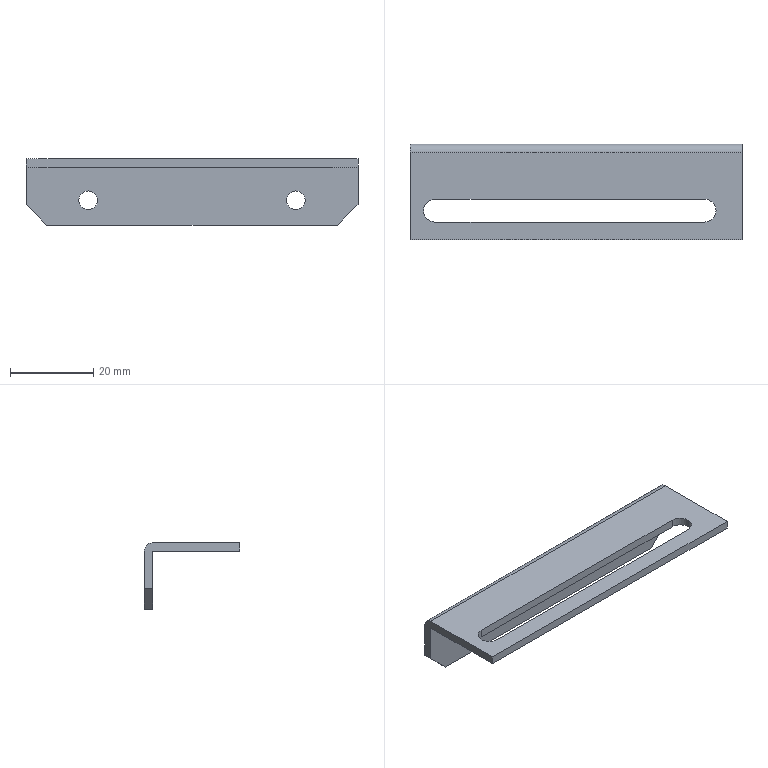Part | SolidWorks | features ICE 5, Chamfer 3, HoleWzd 3, Extrusion 1, Fillet 1 | 1 solid | 20 faces | box 80 x 23 x 16 mm | volume 4975 mm3 | plane 12 | cylinder 8 | commonest cylinder face diameters 4.5 x4 5.5 x3 4 x1
STEP:
#1=CARTESIAN_POINT('',(-10.,10.5,5.75));
#2=VERTEX_POINT('',#1);
#3=CARTESIAN_POINT('',(-10.,10.5,10.25));
#4=VERTEX_POINT('',#3);
#5=CARTESIAN_POINT('',(-10.,10.5,8.));
#6=DIRECTION('',(0.,1.,0.));
#7=DIRECTION('',(0.,0.,1.));
#8=AXIS2_PLACEMENT_3D('',#5,#6,#7);
#9=CIRCLE('',#8,2.25);
#10=EDGE_CURVE('',#2,#4,#9,.T.);
#11=ORIENTED_EDGE('',*,*,#10,.F.);
#12=CARTESIAN_POINT('',(-10.,12.5,5.75));
#13=VERTEX_POINT('',#12);
#14=CARTESIAN_POINT('',(-10.,12.5,5.75));
#15=DIRECTION('',(0.,1.,0.));
#16=VECTOR('',#15,1000.);
#17=LINE('',#14,#16);
#18=EDGE_CURVE('',#2,#13,#17,.T.);
#19=ORIENTED_EDGE('',*,*,#18,.T.);
#20=CARTESIAN_POINT('',(-10.,12.5,10.25));
#21=VERTEX_POINT('',#20);
#22=CARTESIAN_POINT('',(-10.,12.5,8.));
#23=DIRECTION('',(0.,1.,0.));
#24=DIRECTION('',(0.,0.,1.));
#25=AXIS2_PLACEMENT_3D('',#22,#23,#24);
#26=CIRCLE('',#25,2.25);
#27=EDGE_CURVE('',#13,#21,#26,.T.);
#28=ORIENTED_EDGE('',*,*,#27,.T.);
#29=CARTESIAN_POINT('',(-10.,12.5,10.25));
#30=DIRECTION('',(0.,1.,0.));
#31=VECTOR('',#30,1000.);
#32=LINE('',#29,#31);
#33=EDGE_CURVE('',#4,#21,#32,.T.);
#34=ORIENTED_EDGE('',*,*,#33,.F.);
#35=EDGE_LOOP('',(#11,#19,#28,#34));
#36=FACE_OUTER_BOUND('',#35,.T.);
#37=CARTESIAN_POINT('',(-10.,12.5,8.));
#38=DIRECTION('',(0.,1.,0.));
#39=DIRECTION('',(0.,0.,1.));
#40=AXIS2_PLACEMENT_3D('',#37,#38,#39);
#41=CYLINDRICAL_SURFACE('',#40,2.25);
#42=ADVANCED_FACE('',(#36),#41,.F.);
#43=CARTESIAN_POINT('',(-60.,10.5,5.75));
#44=VERTEX_POINT('',#43);
#45=CARTESIAN_POINT('',(-60.,10.5,10.25));
#46=VERTEX_POINT('',#45);
#47=CARTESIAN_POINT('',(-60.,10.5,8.));
#48=DIRECTION('',(0.,1.,0.));
#49=DIRECTION('',(0.,0.,1.));
#50=AXIS2_PLACEMENT_3D('',#47,#48,#49);
#51=CIRCLE('',#50,2.25);
#52=EDGE_CURVE('',#44,#46,#51,.T.);
#53=ORIENTED_EDGE('',*,*,#52,.F.);
#54=CARTESIAN_POINT('',(-60.,12.5,5.75));
#55=VERTEX_POINT('',#54);
#56=CARTESIAN_POINT('',(-60.,12.5,5.75));
#57=DIRECTION('',(0.,1.,0.));
#58=VECTOR('',#57,1000.);
#59=LINE('',#56,#58);
#60=EDGE_CURVE('',#44,#55,#59,.T.);
#61=ORIENTED_EDGE('',*,*,#60,.T.);
#62=CARTESIAN_POINT('',(-60.,12.5,10.25));
#63=VERTEX_POINT('',#62);
#64=CARTESIAN_POINT('',(-60.,12.5,8.));
#65=DIRECTION('',(0.,1.,0.));
#66=DIRECTION('',(0.,0.,1.));
#67=AXIS2_PLACEMENT_3D('',#64,#65,#66);
#68=CIRCLE('',#67,2.25);
#69=EDGE_CURVE('',#55,#63,#68,.T.);
#70=ORIENTED_EDGE('',*,*,#69,.T.);
#71=CARTESIAN_POINT('',(-60.,12.5,10.25));
#72=DIRECTION('',(0.,1.,0.));
#73=VECTOR('',#72,1000.);
#74=LINE('',#71,#73);
#75=EDGE_CURVE('',#46,#63,#74,.T.);
#76=ORIENTED_EDGE('',*,*,#75,.F.);
#77=EDGE_LOOP('',(#53,#61,#70,#76));
#78=FACE_OUTER_BOUND('',#77,.T.);
#79=CARTESIAN_POINT('',(-60.,12.5,8.));
#80=DIRECTION('',(0.,1.,0.));
#81=DIRECTION('',(0.,0.,1.));
#82=AXIS2_PLACEMENT_3D('',#79,#80,#81);
#83=CYLINDRICAL_SURFACE('',#82,2.25);
#84=ADVANCED_FACE('',(#78),#83,.F.);
#85=CARTESIAN_POINT('',(-1.25,-3.5,16.));
#86=VERTEX_POINT('',#85);
#87=CARTESIAN_POINT('',(-4.,-0.75,16.));
#88=VERTEX_POINT('',#87);
#89=CARTESIAN_POINT('',(-4.,-3.5,16.));
#90=DIRECTION('',(0.,0.,1.));
#91=DIRECTION('',(1.,0.,0.));
#92=AXIS2_PLACEMENT_3D('',#89,#90,#91);
#93=CIRCLE('',#92,2.75);
#94=EDGE_CURVE('',#86,#88,#93,.T.);
#95=ORIENTED_EDGE('',*,*,#94,.F.);
#96=CARTESIAN_POINT('',(-1.25,-3.5,18.));
#97=VERTEX_POINT('',#96);
#98=CARTESIAN_POINT('',(-1.25,-3.5,0.));
#99=DIRECTION('',(0.,0.,1.));
#100=VECTOR('',#99,1000.);
#101=LINE('',#98,#100);
#102=EDGE_CURVE('',#86,#97,#101,.T.);
#103=ORIENTED_EDGE('',*,*,#102,.T.);
#104=CARTESIAN_POINT('',(-4.,-0.75,18.));
#105=VERTEX_POINT('',#104);
#106=CARTESIAN_POINT('',(-4.,-3.5,18.));
#107=DIRECTION('',(0.,0.,1.));
#108=DIRECTION('',(1.,0.,0.));
#109=AXIS2_PLACEMENT_3D('',#106,#107,#108);
#110=CIRCLE('',#109,2.75);
#111=EDGE_CURVE('',#97,#105,#110,.T.);
#112=ORIENTED_EDGE('',*,*,#111,.T.);
#113=CARTESIAN_POINT('',(-4.,-0.75,0.));
#114=DIRECTION('',(0.,0.,1.));
#115=VECTOR('',#114,1000.);
#116=LINE('',#113,#115);
#117=EDGE_CURVE('',#88,#105,#116,.T.);
#118=ORIENTED_EDGE('',*,*,#117,.F.);
#119=EDGE_LOOP('',(#95,#103,#112,#118));
#120=FACE_OUTER_BOUND('',#119,.T.);
#121=CARTESIAN_POINT('',(-4.,-3.5,0.));
#122=DIRECTION('',(0.,0.,1.));
#123=DIRECTION('',(1.,0.,0.));
#124=AXIS2_PLACEMENT_3D('',#121,#122,#123);
#125=CYLINDRICAL_SURFACE('',#124,2.75);
#126=ADVANCED_FACE('',(#120),#125,.F.);
#127=CARTESIAN_POINT('',(-75.,-10.5,18.));
#128=VERTEX_POINT('',#127);
#129=CARTESIAN_POINT('',(-75.,-10.5,16.));
#130=VERTEX_POINT('',#129);
#131=CARTESIAN_POINT('',(-75.,-10.5,26.));
#132=DIRECTION('',(0.,0.,-1.));
#133=VECTOR('',#132,1000.);
#134=LINE('',#131,#133);
#135=EDGE_CURVE('',#128,#130,#134,.T.);
#136=ORIENTED_EDGE('',*,*,#135,.F.);
#137=CARTESIAN_POINT('',(-75.,10.5,18.));
#138=VERTEX_POINT('',#137);
#139=CARTESIAN_POINT('',(-75.,-12.5,18.));
#140=DIRECTION('',(0.,1.,0.));
#141=VECTOR('',#140,1000.);
#142=LINE('',#139,#141);
#143=EDGE_CURVE('',#128,#138,#142,.T.);
#144=ORIENTED_EDGE('',*,*,#143,.T.);
#145=CARTESIAN_POINT('',(-75.,12.5,16.));
#146=VERTEX_POINT('',#145);
#147=CARTESIAN_POINT('',(-75.,10.5,16.));
#148=DIRECTION('',(-1.,0.,0.));
#149=DIRECTION('',(0.,0.,1.));
#150=AXIS2_PLACEMENT_3D('',#147,#148,#149);
#151=CIRCLE('',#150,2.);
#152=EDGE_CURVE('',#138,#146,#151,.T.);
#153=ORIENTED_EDGE('',*,*,#152,.T.);
#154=CARTESIAN_POINT('',(-75.,12.5,7.));
#155=VERTEX_POINT('',#154);
#156=CARTESIAN_POINT('',(-75.,12.5,18.));
#157=DIRECTION('',(0.,0.,-1.));
#158=VECTOR('',#157,1000.);
#159=LINE('',#156,#158);
#160=EDGE_CURVE('',#146,#155,#159,.T.);
#161=ORIENTED_EDGE('',*,*,#160,.T.);
#162=CARTESIAN_POINT('',(-75.,10.5,7.));
#163=VERTEX_POINT('',#162);
#164=CARTESIAN_POINT('',(-75.,10.5,7.));
#165=DIRECTION('',(0.,-1.,0.));
#166=VECTOR('',#165,1000.);
#167=LINE('',#164,#166);
#168=EDGE_CURVE('',#155,#163,#167,.T.);
#169=ORIENTED_EDGE('',*,*,#168,.T.);
#170=CARTESIAN_POINT('',(-75.,10.5,16.));
#171=VERTEX_POINT('',#170);
#172=CARTESIAN_POINT('',(-75.,10.5,16.));
#173=DIRECTION('',(0.,0.,-1.));
#174=VECTOR('',#173,1000.);
#175=LINE('',#172,#174);
#176=EDGE_CURVE('',#171,#163,#175,.T.);
#177=ORIENTED_EDGE('',*,*,#176,.F.);
#178=CARTESIAN_POINT('',(-75.,-12.5,16.));
#179=DIRECTION('',(0.,1.,0.));
#180=VECTOR('',#179,1000.);
#181=LINE('',#178,#180);
#182=EDGE_CURVE('',#130,#171,#181,.T.);
#183=ORIENTED_EDGE('',*,*,#182,.F.);
#184=EDGE_LOOP('',(#136,#144,#153,#161,#169,#177,#183));
#185=FACE_OUTER_BOUND('',#184,.T.);
#186=CARTESIAN_POINT('',(-75.,-12.5,18.));
#187=DIRECTION('',(-1.,0.,0.));
#188=DIRECTION('',(0.,0.,1.));
#189=AXIS2_PLACEMENT_3D('',#186,#187,#188);
#190=PLANE('',#189);
#191=ADVANCED_FACE('',(#185),#190,.T.);
#192=CARTESIAN_POINT('',(5.,12.5,7.));
#193=VERTEX_POINT('',#192);
#194=CARTESIAN_POINT('',(5.,12.5,16.));
#195=VERTEX_POINT('',#194);
#196=CARTESIAN_POINT('',(5.,12.5,18.));
#197=DIRECTION('',(0.,0.,1.));
#198=VECTOR('',#197,1000.);
#199=LINE('',#196,#198);
#200=EDGE_CURVE('',#193,#195,#199,.T.);
#201=ORIENTED_EDGE('',*,*,#200,.F.);
#202=CARTESIAN_POINT('',(0.,12.5,2.));
#203=VERTEX_POINT('',#202);
#204=CARTESIAN_POINT('',(-29.5,12.5,-27.5));
#205=DIRECTION('',(-0.7071,0.,-0.7071));
#206=VECTOR('',#205,1000.);
#207=LINE('',#204,#206);
#208=EDGE_CURVE('',#193,#203,#207,.T.);
#209=ORIENTED_EDGE('',*,*,#208,.T.);
#210=CARTESIAN_POINT('',(-70.,12.5,2.));
#211=VERTEX_POINT('',#210);
#212=CARTESIAN_POINT('',(75.,12.5,2.));
#213=DIRECTION('',(1.,0.,0.));
#214=VECTOR('',#213,1000.);
#215=LINE('',#212,#214);
#216=EDGE_CURVE('',#211,#203,#215,.T.);
#217=ORIENTED_EDGE('',*,*,#216,.F.);
#218=CARTESIAN_POINT('',(-80.5,12.5,12.5));
#219=DIRECTION('',(-0.7071,0.,0.7071));
#220=VECTOR('',#219,1000.);
#221=LINE('',#218,#220);
#222=EDGE_CURVE('',#211,#155,#221,.T.);
#223=ORIENTED_EDGE('',*,*,#222,.T.);
#224=ORIENTED_EDGE('',*,*,#160,.F.);
#225=CARTESIAN_POINT('',(75.,12.5,16.));
#226=DIRECTION('',(1.,0.,0.));
#227=VECTOR('',#226,1000.);
#228=LINE('',#225,#227);
#229=EDGE_CURVE('',#146,#195,#228,.T.);
#230=ORIENTED_EDGE('',*,*,#229,.T.);
#231=EDGE_LOOP('',(#201,#209,#217,#223,#224,#230));
#232=FACE_OUTER_BOUND('',#231,.T.);
#233=CARTESIAN_POINT('',(-10.,12.5,8.));
#234=DIRECTION('',(0.,1.,0.));
#235=DIRECTION('',(0.,0.,1.));
#236=AXIS2_PLACEMENT_3D('',#233,#234,#235);
#237=CIRCLE('',#236,2.25);
#238=EDGE_CURVE('',#21,#13,#237,.T.);
#239=ORIENTED_EDGE('',*,*,#238,.F.);
#240=ORIENTED_EDGE('',*,*,#27,.F.);
#241=EDGE_LOOP('',(#239,#240));
#242=FACE_BOUND('',#241,.T.);
#243=CARTESIAN_POINT('',(-60.,12.5,8.));
#244=DIRECTION('',(0.,1.,0.));
#245=DIRECTION('',(0.,0.,1.));
#246=AXIS2_PLACEMENT_3D('',#243,#244,#245);
#247=CIRCLE('',#246,2.25);
#248=EDGE_CURVE('',#63,#55,#247,.T.);
#249=ORIENTED_EDGE('',*,*,#248,.F.);
#250=ORIENTED_EDGE('',*,*,#69,.F.);
#251=EDGE_LOOP('',(#249,#250));
#252=FACE_BOUND('',#251,.T.);
#253=CARTESIAN_POINT('',(-75.,12.5,18.));
#254=DIRECTION('',(0.,1.,0.));
#255=DIRECTION('',(0.,0.,1.));
#256=AXIS2_PLACEMENT_3D('',#253,#254,#255);
#257=PLANE('',#256);
#258=ADVANCED_FACE('',(#232,#242,#252),#257,.T.);
#259=CARTESIAN_POINT('',(-69.,-6.25,18.));
#260=VERTEX_POINT('',#259);
#261=CARTESIAN_POINT('',(-4.,-6.25,18.));
#262=VERTEX_POINT('',#261);
#263=CARTESIAN_POINT('',(-69.,-6.25,18.));
#264=DIRECTION('',(1.,0.,0.));
#265=VECTOR('',#264,1000.);
#266=LINE('',#263,#265);
#267=EDGE_CURVE('',#260,#262,#266,.T.);
#268=ORIENTED_EDGE('',*,*,#267,.F.);
#269=CARTESIAN_POINT('',(-69.,-0.75,18.));
#270=VERTEX_POINT('',#269);
#271=CARTESIAN_POINT('',(-69.,-3.5,18.));
#272=DIRECTION('',(0.,0.,1.));
#273=DIRECTION('',(1.,0.,0.));
#274=AXIS2_PLACEMENT_3D('',#271,#272,#273);
#275=CIRCLE('',#274,2.75);
#276=EDGE_CURVE('',#270,#260,#275,.T.);
#277=ORIENTED_EDGE('',*,*,#276,.F.);
#278=CARTESIAN_POINT('',(-4.,-0.75,18.));
#279=DIRECTION('',(-1.,0.,0.));
#280=VECTOR('',#279,1000.);
#281=LINE('',#278,#280);
#282=EDGE_CURVE('',#105,#270,#281,.T.);
#283=ORIENTED_EDGE('',*,*,#282,.F.);
#284=ORIENTED_EDGE('',*,*,#111,.F.);
#285=CARTESIAN_POINT('',(-4.,-3.5,18.));
#286=DIRECTION('',(0.,0.,1.));
#287=DIRECTION('',(1.,0.,0.));
#288=AXIS2_PLACEMENT_3D('',#285,#286,#287);
#289=CIRCLE('',#288,2.75);
#290=EDGE_CURVE('',#262,#97,#289,.T.);
#291=ORIENTED_EDGE('',*,*,#290,.F.);
#292=EDGE_LOOP('',(#268,#277,#283,#284,#291));
#293=FACE_BOUND('',#292,.T.);
#294=ORIENTED_EDGE('',*,*,#143,.F.);
#295=CARTESIAN_POINT('',(5.,-10.5,18.));
#296=VERTEX_POINT('',#295);
#297=CARTESIAN_POINT('',(-75.,-10.5,18.));
#298=DIRECTION('',(1.,0.,0.));
#299=VECTOR('',#298,1000.);
#300=LINE('',#297,#299);
#301=EDGE_CURVE('',#128,#296,#300,.T.);
#302=ORIENTED_EDGE('',*,*,#301,.T.);
#303=CARTESIAN_POINT('',(5.,10.5,18.));
#304=VERTEX_POINT('',#303);
#305=CARTESIAN_POINT('',(5.,-22.929,18.));
#306=DIRECTION('',(0.,1.,0.));
#307=VECTOR('',#306,1000.);
#308=LINE('',#305,#307);
#309=EDGE_CURVE('',#296,#304,#308,.T.);
#310=ORIENTED_EDGE('',*,*,#309,.T.);
#311=CARTESIAN_POINT('',(-75.,10.5,18.));
#312=DIRECTION('',(-1.,0.,0.));
#313=VECTOR('',#312,1000.);
#314=LINE('',#311,#313);
#315=EDGE_CURVE('',#304,#138,#314,.T.);
#316=ORIENTED_EDGE('',*,*,#315,.T.);
#317=EDGE_LOOP('',(#294,#302,#310,#316));
#318=FACE_OUTER_BOUND('',#317,.T.);
#319=CARTESIAN_POINT('',(-75.,12.5,18.));
#320=DIRECTION('',(0.,0.,-1.));
#321=DIRECTION('',(-1.,0.,0.));
#322=AXIS2_PLACEMENT_3D('',#319,#320,#321);
#323=PLANE('',#322);
#324=ADVANCED_FACE('',(#293,#318),#323,.F.);
#325=CARTESIAN_POINT('',(-10.,10.5,8.));
#326=DIRECTION('',(0.,1.,0.));
#327=DIRECTION('',(0.,0.,1.));
#328=AXIS2_PLACEMENT_3D('',#325,#326,#327);
#329=CIRCLE('',#328,2.25);
#330=EDGE_CURVE('',#4,#2,#329,.T.);
#331=ORIENTED_EDGE('',*,*,#330,.T.);
#332=ORIENTED_EDGE('',*,*,#10,.T.);
#333=EDGE_LOOP('',(#331,#332));
#334=FACE_BOUND('',#333,.T.);
#335=CARTESIAN_POINT('',(-60.,10.5,8.));
#336=DIRECTION('',(0.,1.,0.));
#337=DIRECTION('',(0.,0.,1.));
#338=AXIS2_PLACEMENT_3D('',#335,#336,#337);
#339=CIRCLE('',#338,2.25);
#340=EDGE_CURVE('',#46,#44,#339,.T.);
#341=ORIENTED_EDGE('',*,*,#340,.T.);
#342=ORIENTED_EDGE('',*,*,#52,.T.);
#343=EDGE_LOOP('',(#341,#342));
#344=FACE_BOUND('',#343,.T.);
#345=CARTESIAN_POINT('',(-70.,10.5,2.));
#346=VERTEX_POINT('',#345);
#347=CARTESIAN_POINT('',(0.,10.5,2.));
#348=VERTEX_POINT('',#347);
#349=CARTESIAN_POINT('',(75.,10.5,2.));
#350=DIRECTION('',(1.,0.,0.));
#351=VECTOR('',#350,1000.);
#352=LINE('',#349,#351);
#353=EDGE_CURVE('',#346,#348,#352,.T.);
#354=ORIENTED_EDGE('',*,*,#353,.T.);
#355=CARTESIAN_POINT('',(5.,10.5,7.));
#356=VERTEX_POINT('',#355);
#357=CARTESIAN_POINT('',(5.,10.5,7.));
#358=DIRECTION('',(0.7071,0.,0.7071));
#359=VECTOR('',#358,1000.);
#360=LINE('',#357,#359);
#361=EDGE_CURVE('',#348,#356,#360,.T.);
#362=ORIENTED_EDGE('',*,*,#361,.T.);
#363=CARTESIAN_POINT('',(5.,10.5,16.));
#364=VERTEX_POINT('',#363);
#365=CARTESIAN_POINT('',(5.,10.5,16.));
#366=DIRECTION('',(0.,0.,1.));
#367=VECTOR('',#366,1000.);
#368=LINE('',#365,#367);
#369=EDGE_CURVE('',#356,#364,#368,.T.);
#370=ORIENTED_EDGE('',*,*,#369,.T.);
#371=CARTESIAN_POINT('',(75.,10.5,16.));
#372=DIRECTION('',(-1.,0.,0.));
#373=VECTOR('',#372,1000.);
#374=LINE('',#371,#373);
#375=EDGE_CURVE('',#364,#171,#374,.T.);
#376=ORIENTED_EDGE('',*,*,#375,.T.);
#377=ORIENTED_EDGE('',*,*,#176,.T.);
#378=CARTESIAN_POINT('',(-70.,10.5,2.));
#379=DIRECTION('',(0.7071,0.,-0.7071));
#380=VECTOR('',#379,1000.);
#381=LINE('',#378,#380);
#382=EDGE_CURVE('',#163,#346,#381,.T.);
#383=ORIENTED_EDGE('',*,*,#382,.T.);
#384=EDGE_LOOP('',(#354,#362,#370,#376,#377,#383));
#385=FACE_OUTER_BOUND('',#384,.T.);
#386=CARTESIAN_POINT('',(75.,10.5,16.));
#387=DIRECTION('',(0.,1.,0.));
#388=DIRECTION('',(0.,0.,1.));
#389=AXIS2_PLACEMENT_3D('',#386,#387,#388);
#390=PLANE('',#389);
#391=ADVANCED_FACE('',(#334,#344,#385),#390,.F.);
#392=CARTESIAN_POINT('',(-69.,-0.75,16.));
#393=VERTEX_POINT('',#392);
#394=CARTESIAN_POINT('',(75.,-0.75,16.));
#395=DIRECTION('',(-1.,0.,0.));
#396=VECTOR('',#395,1000.);
#397=LINE('',#394,#396);
#398=EDGE_CURVE('',#88,#393,#397,.T.);
#399=ORIENTED_EDGE('',*,*,#398,.T.);
#400=CARTESIAN_POINT('',(-69.,-6.25,16.));
#401=VERTEX_POINT('',#400);
#402=CARTESIAN_POINT('',(-69.,-3.5,16.));
#403=DIRECTION('',(0.,0.,1.));
#404=DIRECTION('',(1.,0.,0.));
#405=AXIS2_PLACEMENT_3D('',#402,#403,#404);
#406=CIRCLE('',#405,2.75);
#407=EDGE_CURVE('',#393,#401,#406,.T.);
#408=ORIENTED_EDGE('',*,*,#407,.T.);
#409=CARTESIAN_POINT('',(-4.,-6.25,16.));
#410=VERTEX_POINT('',#409);
#411=CARTESIAN_POINT('',(75.,-6.25,16.));
#412=DIRECTION('',(1.,0.,0.));
#413=VECTOR('',#412,1000.);
#414=LINE('',#411,#413);
#415=EDGE_CURVE('',#401,#410,#414,.T.);
#416=ORIENTED_EDGE('',*,*,#415,.T.);
#417=CARTESIAN_POINT('',(-4.,-3.5,16.));
#418=DIRECTION('',(0.,0.,1.));
#419=DIRECTION('',(1.,0.,0.));
#420=AXIS2_PLACEMENT_3D('',#417,#418,#419);
#421=CIRCLE('',#420,2.75);
#422=EDGE_CURVE('',#410,#86,#421,.T.);
#423=ORIENTED_EDGE('',*,*,#422,.T.);
#424=ORIENTED_EDGE('',*,*,#94,.T.);
#425=EDGE_LOOP('',(#399,#408,#416,#423,#424));
#426=FACE_BOUND('',#425,.T.);
#427=CARTESIAN_POINT('',(5.,-10.5,16.));
#428=VERTEX_POINT('',#427);
#429=CARTESIAN_POINT('',(5.,-12.5,16.));
#430=DIRECTION('',(0.,-1.,0.));
#431=VECTOR('',#430,1000.);
#432=LINE('',#429,#431);
#433=EDGE_CURVE('',#364,#428,#432,.T.);
#434=ORIENTED_EDGE('',*,*,#433,.T.);
#435=CARTESIAN_POINT('',(-75.,-10.5,16.));
#436=DIRECTION('',(1.,0.,0.));
#437=VECTOR('',#436,1000.);
#438=LINE('',#435,#437);
#439=EDGE_CURVE('',#130,#428,#438,.T.);
#440=ORIENTED_EDGE('',*,*,#439,.F.);
#441=ORIENTED_EDGE('',*,*,#182,.T.);
#442=ORIENTED_EDGE('',*,*,#375,.F.);
#443=EDGE_LOOP('',(#434,#440,#441,#442));
#444=FACE_OUTER_BOUND('',#443,.T.);
#445=CARTESIAN_POINT('',(75.,-12.5,16.));
#446=DIRECTION('',(0.,0.,1.));
#447=DIRECTION('',(1.,0.,0.));
#448=AXIS2_PLACEMENT_3D('',#445,#446,#447);
#449=PLANE('',#448);
#450=ADVANCED_FACE('',(#426,#444),#449,.F.);
#451=CARTESIAN_POINT('',(-69.,-0.75,0.));
#452=DIRECTION('',(0.,0.,1.));
#453=VECTOR('',#452,1000.);
#454=LINE('',#451,#453);
#455=EDGE_CURVE('',#393,#270,#454,.T.);
#456=ORIENTED_EDGE('',*,*,#455,.T.);
#457=ORIENTED_EDGE('',*,*,#276,.T.);
#458=CARTESIAN_POINT('',(-69.,-6.25,0.));
#459=DIRECTION('',(0.,0.,1.));
#460=VECTOR('',#459,1000.);
#461=LINE('',#458,#460);
#462=EDGE_CURVE('',#401,#260,#461,.T.);
#463=ORIENTED_EDGE('',*,*,#462,.F.);
#464=ORIENTED_EDGE('',*,*,#407,.F.);
#465=EDGE_LOOP('',(#456,#457,#463,#464));
#466=FACE_OUTER_BOUND('',#465,.T.);
#467=CARTESIAN_POINT('',(-69.,-3.5,0.));
#468=DIRECTION('',(0.,0.,1.));
#469=DIRECTION('',(1.,0.,0.));
#470=AXIS2_PLACEMENT_3D('',#467,#468,#469);
#471=CYLINDRICAL_SURFACE('',#470,2.75);
#472=ADVANCED_FACE('',(#466),#471,.F.);
#473=ORIENTED_EDGE('',*,*,#117,.T.);
#474=ORIENTED_EDGE('',*,*,#282,.T.);
#475=ORIENTED_EDGE('',*,*,#455,.F.);
#476=ORIENTED_EDGE('',*,*,#398,.F.);
#477=EDGE_LOOP('',(#473,#474,#475,#476));
#478=FACE_OUTER_BOUND('',#477,.T.);
#479=CARTESIAN_POINT('',(-4.,-0.75,0.));
#480=DIRECTION('',(0.,1.,0.));
#481=DIRECTION('',(-1.,0.,0.));
#482=AXIS2_PLACEMENT_3D('',#479,#480,#481);
#483=PLANE('',#482);
#484=ADVANCED_FACE('',(#478),#483,.F.);
#485=ORIENTED_EDGE('',*,*,#102,.F.);
#486=ORIENTED_EDGE('',*,*,#422,.F.);
#487=CARTESIAN_POINT('',(-4.,-6.25,0.));
#488=DIRECTION('',(0.,0.,1.));
#489=VECTOR('',#488,1000.);
#490=LINE('',#487,#489);
#491=EDGE_CURVE('',#410,#262,#490,.T.);
#492=ORIENTED_EDGE('',*,*,#491,.T.);
#493=ORIENTED_EDGE('',*,*,#290,.T.);
#494=EDGE_LOOP('',(#485,#486,#492,#493));
#495=FACE_OUTER_BOUND('',#494,.T.);
#496=CARTESIAN_POINT('',(-4.,-3.5,0.));
#497=DIRECTION('',(0.,0.,1.));
#498=DIRECTION('',(1.,0.,0.));
#499=AXIS2_PLACEMENT_3D('',#496,#497,#498);
#500=CYLINDRICAL_SURFACE('',#499,2.75);
#501=ADVANCED_FACE('',(#495),#500,.F.);
#502=ORIENTED_EDGE('',*,*,#462,.T.);
#503=ORIENTED_EDGE('',*,*,#267,.T.);
#504=ORIENTED_EDGE('',*,*,#491,.F.);
#505=ORIENTED_EDGE('',*,*,#415,.F.);
#506=EDGE_LOOP('',(#502,#503,#504,#505));
#507=FACE_OUTER_BOUND('',#506,.T.);
#508=CARTESIAN_POINT('',(-69.,-6.25,0.));
#509=DIRECTION('',(0.,-1.,0.));
#510=DIRECTION('',(0.,0.,-1.));
#511=AXIS2_PLACEMENT_3D('',#508,#509,#510);
#512=PLANE('',#511);
#513=ADVANCED_FACE('',(#507),#512,.F.);
#514=ORIENTED_EDGE('',*,*,#60,.F.);
#515=ORIENTED_EDGE('',*,*,#340,.F.);
#516=ORIENTED_EDGE('',*,*,#75,.T.);
#517=ORIENTED_EDGE('',*,*,#248,.T.);
#518=EDGE_LOOP('',(#514,#515,#516,#517));
#519=FACE_OUTER_BOUND('',#518,.T.);
#520=CARTESIAN_POINT('',(-60.,12.5,8.));
#521=DIRECTION('',(0.,1.,0.));
#522=DIRECTION('',(0.,0.,1.));
#523=AXIS2_PLACEMENT_3D('',#520,#521,#522);
#524=CYLINDRICAL_SURFACE('',#523,2.25);
#525=ADVANCED_FACE('',(#519),#524,.F.);
#526=ORIENTED_EDGE('',*,*,#18,.F.);
#527=ORIENTED_EDGE('',*,*,#330,.F.);
#528=ORIENTED_EDGE('',*,*,#33,.T.);
#529=ORIENTED_EDGE('',*,*,#238,.T.);
#530=EDGE_LOOP('',(#526,#527,#528,#529));
#531=FACE_OUTER_BOUND('',#530,.T.);
#532=CARTESIAN_POINT('',(-10.,12.5,8.));
#533=DIRECTION('',(0.,1.,0.));
#534=DIRECTION('',(0.,0.,1.));
#535=AXIS2_PLACEMENT_3D('',#532,#533,#534);
#536=CYLINDRICAL_SURFACE('',#535,2.25);
#537=ADVANCED_FACE('',(#531),#536,.F.);
#538=CARTESIAN_POINT('',(5.,10.5,16.));
#539=DIRECTION('',(1.,0.,0.));
#540=DIRECTION('',(0.,0.,1.));
#541=AXIS2_PLACEMENT_3D('',#538,#539,#540);
#542=CIRCLE('',#541,2.);
#543=EDGE_CURVE('',#195,#304,#542,.T.);
#544=ORIENTED_EDGE('',*,*,#543,.F.);
#545=ORIENTED_EDGE('',*,*,#229,.F.);
#546=ORIENTED_EDGE('',*,*,#152,.F.);
#547=ORIENTED_EDGE('',*,*,#315,.F.);
#548=EDGE_LOOP('',(#544,#545,#546,#547));
#549=FACE_OUTER_BOUND('',#548,.T.);
#550=CARTESIAN_POINT('',(-75.,10.5,16.));
#551=DIRECTION('',(-1.,0.,0.));
#552=DIRECTION('',(0.,0.,1.));
#553=AXIS2_PLACEMENT_3D('',#550,#551,#552);
#554=CYLINDRICAL_SURFACE('',#553,2.);
#555=ADVANCED_FACE('',(#549),#554,.T.);
#556=ORIENTED_EDGE('',*,*,#216,.T.);
#557=CARTESIAN_POINT('',(0.,2.5,2.));
#558=DIRECTION('',(0.,-1.,0.));
#559=VECTOR('',#558,1000.);
#560=LINE('',#557,#559);
#561=EDGE_CURVE('',#203,#348,#560,.T.);
#562=ORIENTED_EDGE('',*,*,#561,.T.);
#563=ORIENTED_EDGE('',*,*,#353,.F.);
#564=CARTESIAN_POINT('',(-70.,12.5,2.));
#565=DIRECTION('',(0.,1.,0.));
#566=VECTOR('',#565,1000.);
#567=LINE('',#564,#566);
#568=EDGE_CURVE('',#346,#211,#567,.T.);
#569=ORIENTED_EDGE('',*,*,#568,.T.);
#570=EDGE_LOOP('',(#556,#562,#563,#569));
#571=FACE_OUTER_BOUND('',#570,.T.);
#572=CARTESIAN_POINT('',(75.,2.5,2.));
#573=DIRECTION('',(0.,0.,1.));
#574=DIRECTION('',(1.,0.,0.));
#575=AXIS2_PLACEMENT_3D('',#572,#573,#574);
#576=PLANE('',#575);
#577=ADVANCED_FACE('',(#571),#576,.F.);
#578=ORIENTED_EDGE('',*,*,#382,.F.);
#579=ORIENTED_EDGE('',*,*,#168,.F.);
#580=ORIENTED_EDGE('',*,*,#222,.F.);
#581=ORIENTED_EDGE('',*,*,#568,.F.);
#582=EDGE_LOOP('',(#578,#579,#580,#581));
#583=FACE_OUTER_BOUND('',#582,.T.);
#584=CARTESIAN_POINT('',(-70.,2.5,2.));
#585=DIRECTION('',(-0.7071,0.,-0.7071));
#586=DIRECTION('',(-0.7071,0.,0.7071));
#587=AXIS2_PLACEMENT_3D('',#584,#585,#586);
#588=PLANE('',#587);
#589=ADVANCED_FACE('',(#583),#588,.T.);
#590=ORIENTED_EDGE('',*,*,#309,.F.);
#591=CARTESIAN_POINT('',(5.,-10.5,18.));
#592=DIRECTION('',(0.,0.,-1.));
#593=VECTOR('',#592,1000.);
#594=LINE('',#591,#593);
#595=EDGE_CURVE('',#296,#428,#594,.T.);
#596=ORIENTED_EDGE('',*,*,#595,.T.);
#597=ORIENTED_EDGE('',*,*,#433,.F.);
#598=ORIENTED_EDGE('',*,*,#369,.F.);
#599=CARTESIAN_POINT('',(5.,-22.929,7.));
#600=DIRECTION('',(0.,1.,0.));
#601=VECTOR('',#600,1000.);
#602=LINE('',#599,#601);
#603=EDGE_CURVE('',#356,#193,#602,.T.);
#604=ORIENTED_EDGE('',*,*,#603,.T.);
#605=ORIENTED_EDGE('',*,*,#200,.T.);
#606=ORIENTED_EDGE('',*,*,#543,.T.);
#607=EDGE_LOOP('',(#590,#596,#597,#598,#604,#605,#606));
#608=FACE_OUTER_BOUND('',#607,.T.);
#609=CARTESIAN_POINT('',(5.,-22.929,18.));
#610=DIRECTION('',(-1.,0.,0.));
#611=DIRECTION('',(0.,0.,1.));
#612=AXIS2_PLACEMENT_3D('',#609,#610,#611);
#613=PLANE('',#612);
#614=ADVANCED_FACE('',(#608),#613,.F.);
#615=ORIENTED_EDGE('',*,*,#361,.F.);
#616=ORIENTED_EDGE('',*,*,#561,.F.);
#617=ORIENTED_EDGE('',*,*,#208,.F.);
#618=ORIENTED_EDGE('',*,*,#603,.F.);
#619=EDGE_LOOP('',(#615,#616,#617,#618));
#620=FACE_OUTER_BOUND('',#619,.T.);
#621=CARTESIAN_POINT('',(5.,-22.929,7.));
#622=DIRECTION('',(-0.7071,0.,0.7071));
#623=DIRECTION('',(0.7071,0.,0.7071));
#624=AXIS2_PLACEMENT_3D('',#621,#622,#623);
#625=PLANE('',#624);
#626=ADVANCED_FACE('',(#620),#625,.F.);
#627=ORIENTED_EDGE('',*,*,#135,.T.);
#628=ORIENTED_EDGE('',*,*,#439,.T.);
#629=ORIENTED_EDGE('',*,*,#595,.F.);
#630=ORIENTED_EDGE('',*,*,#301,.F.);
#631=EDGE_LOOP('',(#627,#628,#629,#630));
#632=FACE_OUTER_BOUND('',#631,.T.);
#633=CARTESIAN_POINT('',(-75.,-10.5,26.));
#634=DIRECTION('',(0.,1.,0.));
#635=DIRECTION('',(-1.,0.,0.));
#636=AXIS2_PLACEMENT_3D('',#633,#634,#635);
#637=PLANE('',#636);
#638=ADVANCED_FACE('',(#632),#637,.F.);
#639=CLOSED_SHELL('',(#42,#84,#126,#191,#258,#324,#391,#450,#472,#484,#501,#513,#525,#537,#555,#577,#589,#614,#626,#638));
#640=MANIFOLD_SOLID_BREP('',#639);
#641=CARTESIAN_POINT('',(0.,0.,0.));
#642=DIRECTION('',(0.,0.,1.));
#643=DIRECTION('',(1.,0.,0.));
#644=AXIS2_PLACEMENT_3D('',#641,#642,#643);
#645=(LENGTH_UNIT()NAMED_UNIT(*)SI_UNIT(.MILLI.,.METRE.));
#646=UNCERTAINTY_MEASURE_WITH_UNIT(LENGTH_MEASURE(0.00001),#645,'','');
#647=(NAMED_UNIT(*)PLANE_ANGLE_UNIT()SI_UNIT($,.RADIAN.));
#648=(NAMED_UNIT(*)SI_UNIT($,.STERADIAN.)SOLID_ANGLE_UNIT());
#649=(GEOMETRIC_REPRESENTATION_CONTEXT(3)GLOBAL_UNCERTAINTY_ASSIGNED_CONTEXT((#646))GLOBAL_UNIT_ASSIGNED_CONTEXT((#645,#647,#648))REPRESENTATION_CONTEXT('',''));
#650=ADVANCED_BREP_SHAPE_REPRESENTATION('',(#640,#644),#649);